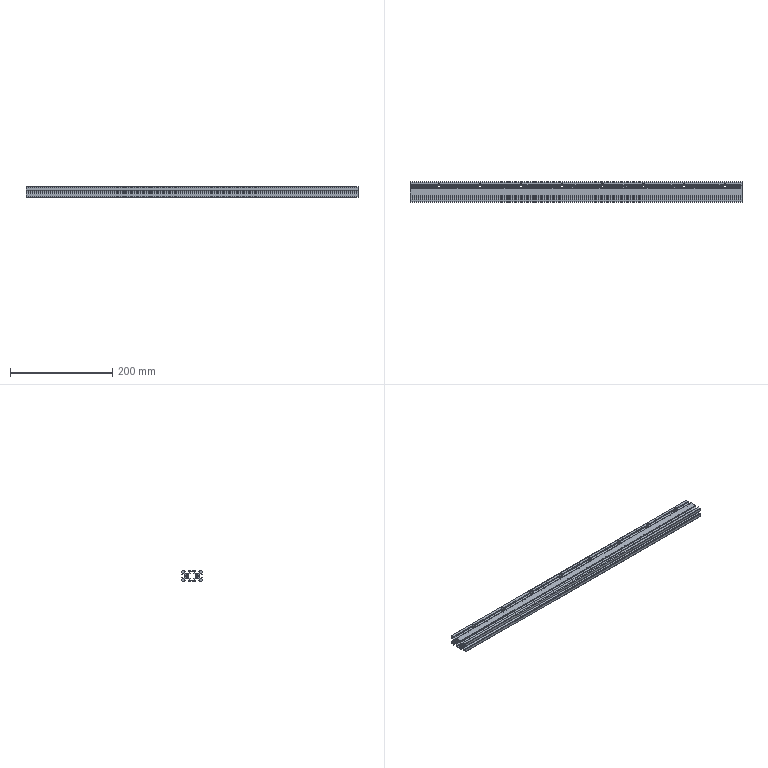Part | STEP file | PN_0005_default[machined] | 1 solid | 390 faces | box 650 x 40 x 20 mm | volume 192154 mm3 | plane 302 | cylinder 88 | commonest cylinder face diameters 10 x48 5.5 x24 5 x12 2 x4